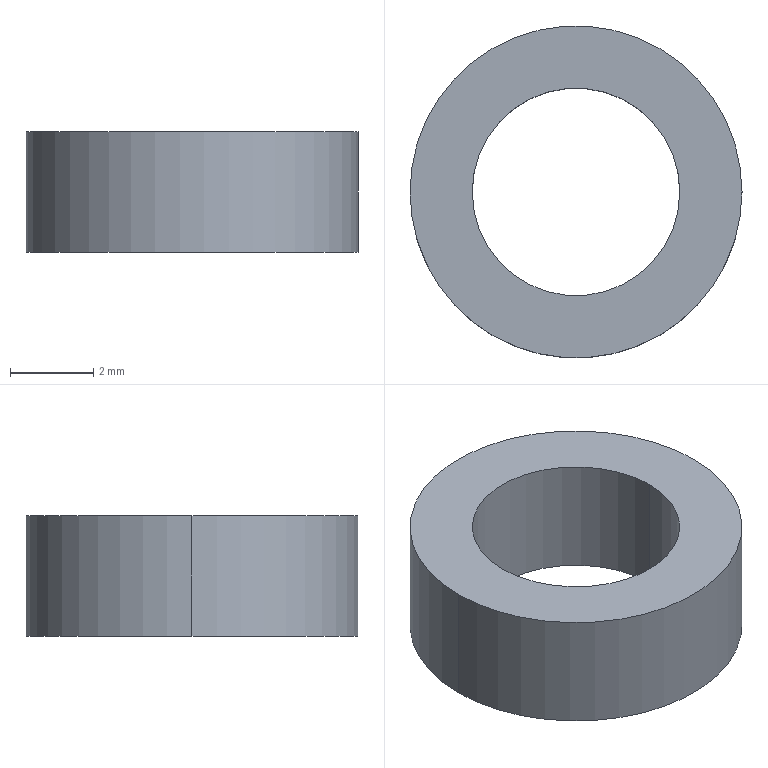Part | SolidWorks | features Extrusion 1 | 1 solid | 6 faces | box 8 x 8 x 2.9 mm | volume 88.829 mm3 | cylinder 4 | plane 2 | commonest cylinder face diameters 5 x2 8 x2
STEP:
#1=CARTESIAN_POINT('',(-2.5,0.,2.9));
#2=VERTEX_POINT('',#1);
#3=CARTESIAN_POINT('',(2.5,0.,2.9));
#4=VERTEX_POINT('',#3);
#5=CARTESIAN_POINT('',(0.,0.,2.9));
#6=DIRECTION('',(0.,0.,1.));
#7=DIRECTION('',(1.,0.,0.));
#8=AXIS2_PLACEMENT_3D('',#5,#6,#7);
#9=CIRCLE('',#8,2.5);
#10=EDGE_CURVE('',#2,#4,#9,.T.);
#11=ORIENTED_EDGE('',*,*,#10,.T.);
#12=CARTESIAN_POINT('',(2.5,0.,0.));
#13=VERTEX_POINT('',#12);
#14=CARTESIAN_POINT('',(2.5,0.,2.9));
#15=DIRECTION('',(0.,0.,-1.));
#16=VECTOR('',#15,1000.);
#17=LINE('',#14,#16);
#18=EDGE_CURVE('',#4,#13,#17,.T.);
#19=ORIENTED_EDGE('',*,*,#18,.T.);
#20=CARTESIAN_POINT('',(-2.5,0.,0.));
#21=VERTEX_POINT('',#20);
#22=CARTESIAN_POINT('',(0.,0.,0.));
#23=DIRECTION('',(0.,0.,1.));
#24=DIRECTION('',(1.,0.,0.));
#25=AXIS2_PLACEMENT_3D('',#22,#23,#24);
#26=CIRCLE('',#25,2.5);
#27=EDGE_CURVE('',#21,#13,#26,.T.);
#28=ORIENTED_EDGE('',*,*,#27,.F.);
#29=CARTESIAN_POINT('',(-2.5,0.,2.9));
#30=DIRECTION('',(0.,0.,-1.));
#31=VECTOR('',#30,1000.);
#32=LINE('',#29,#31);
#33=EDGE_CURVE('',#2,#21,#32,.T.);
#34=ORIENTED_EDGE('',*,*,#33,.F.);
#35=EDGE_LOOP('',(#11,#19,#28,#34));
#36=FACE_OUTER_BOUND('',#35,.T.);
#37=CARTESIAN_POINT('',(0.,0.,2.9));
#38=DIRECTION('',(0.,0.,-1.));
#39=DIRECTION('',(-1.,0.,0.));
#40=AXIS2_PLACEMENT_3D('',#37,#38,#39);
#41=CYLINDRICAL_SURFACE('',#40,2.5);
#42=ADVANCED_FACE('',(#36),#41,.F.);
#43=CARTESIAN_POINT('',(4.,0.,2.9));
#44=VERTEX_POINT('',#43);
#45=CARTESIAN_POINT('',(-4.,0.,2.9));
#46=VERTEX_POINT('',#45);
#47=CARTESIAN_POINT('',(0.,0.,2.9));
#48=DIRECTION('',(0.,0.,1.));
#49=DIRECTION('',(1.,0.,0.));
#50=AXIS2_PLACEMENT_3D('',#47,#48,#49);
#51=CIRCLE('',#50,4.);
#52=EDGE_CURVE('',#44,#46,#51,.T.);
#53=ORIENTED_EDGE('',*,*,#52,.F.);
#54=CARTESIAN_POINT('',(4.,0.,0.));
#55=VERTEX_POINT('',#54);
#56=CARTESIAN_POINT('',(4.,0.,2.9));
#57=DIRECTION('',(0.,0.,-1.));
#58=VECTOR('',#57,1000.);
#59=LINE('',#56,#58);
#60=EDGE_CURVE('',#44,#55,#59,.T.);
#61=ORIENTED_EDGE('',*,*,#60,.T.);
#62=CARTESIAN_POINT('',(-4.,0.,0.));
#63=VERTEX_POINT('',#62);
#64=CARTESIAN_POINT('',(0.,0.,0.));
#65=DIRECTION('',(0.,0.,1.));
#66=DIRECTION('',(1.,0.,0.));
#67=AXIS2_PLACEMENT_3D('',#64,#65,#66);
#68=CIRCLE('',#67,4.);
#69=EDGE_CURVE('',#55,#63,#68,.T.);
#70=ORIENTED_EDGE('',*,*,#69,.T.);
#71=CARTESIAN_POINT('',(-4.,0.,2.9));
#72=DIRECTION('',(0.,0.,-1.));
#73=VECTOR('',#72,1000.);
#74=LINE('',#71,#73);
#75=EDGE_CURVE('',#46,#63,#74,.T.);
#76=ORIENTED_EDGE('',*,*,#75,.F.);
#77=EDGE_LOOP('',(#53,#61,#70,#76));
#78=FACE_OUTER_BOUND('',#77,.T.);
#79=CARTESIAN_POINT('',(0.,0.,2.9));
#80=DIRECTION('',(0.,0.,-1.));
#81=DIRECTION('',(-1.,0.,0.));
#82=AXIS2_PLACEMENT_3D('',#79,#80,#81);
#83=CYLINDRICAL_SURFACE('',#82,4.);
#84=ADVANCED_FACE('',(#78),#83,.T.);
#85=CARTESIAN_POINT('',(0.,0.,2.9));
#86=DIRECTION('',(0.,0.,1.));
#87=DIRECTION('',(1.,0.,0.));
#88=AXIS2_PLACEMENT_3D('',#85,#86,#87);
#89=CIRCLE('',#88,4.);
#90=EDGE_CURVE('',#46,#44,#89,.T.);
#91=ORIENTED_EDGE('',*,*,#90,.T.);
#92=ORIENTED_EDGE('',*,*,#52,.T.);
#93=EDGE_LOOP('',(#91,#92));
#94=FACE_OUTER_BOUND('',#93,.T.);
#95=ORIENTED_EDGE('',*,*,#10,.F.);
#96=CARTESIAN_POINT('',(0.,0.,2.9));
#97=DIRECTION('',(0.,0.,1.));
#98=DIRECTION('',(1.,0.,0.));
#99=AXIS2_PLACEMENT_3D('',#96,#97,#98);
#100=CIRCLE('',#99,2.5);
#101=EDGE_CURVE('',#4,#2,#100,.T.);
#102=ORIENTED_EDGE('',*,*,#101,.F.);
#103=EDGE_LOOP('',(#95,#102));
#104=FACE_BOUND('',#103,.T.);
#105=CARTESIAN_POINT('',(0.,0.,2.9));
#106=DIRECTION('',(0.,0.,1.));
#107=DIRECTION('',(1.,0.,0.));
#108=AXIS2_PLACEMENT_3D('',#105,#106,#107);
#109=PLANE('',#108);
#110=ADVANCED_FACE('',(#94,#104),#109,.T.);
#111=CARTESIAN_POINT('',(0.,0.,0.));
#112=DIRECTION('',(0.,0.,1.));
#113=DIRECTION('',(1.,0.,0.));
#114=AXIS2_PLACEMENT_3D('',#111,#112,#113);
#115=CIRCLE('',#114,4.);
#116=EDGE_CURVE('',#63,#55,#115,.T.);
#117=ORIENTED_EDGE('',*,*,#116,.F.);
#118=ORIENTED_EDGE('',*,*,#69,.F.);
#119=EDGE_LOOP('',(#117,#118));
#120=FACE_OUTER_BOUND('',#119,.T.);
#121=ORIENTED_EDGE('',*,*,#27,.T.);
#122=CARTESIAN_POINT('',(0.,0.,0.));
#123=DIRECTION('',(0.,0.,1.));
#124=DIRECTION('',(1.,0.,0.));
#125=AXIS2_PLACEMENT_3D('',#122,#123,#124);
#126=CIRCLE('',#125,2.5);
#127=EDGE_CURVE('',#13,#21,#126,.T.);
#128=ORIENTED_EDGE('',*,*,#127,.T.);
#129=EDGE_LOOP('',(#121,#128));
#130=FACE_BOUND('',#129,.T.);
#131=CARTESIAN_POINT('',(0.,0.,0.));
#132=DIRECTION('',(0.,0.,1.));
#133=DIRECTION('',(1.,0.,0.));
#134=AXIS2_PLACEMENT_3D('',#131,#132,#133);
#135=PLANE('',#134);
#136=ADVANCED_FACE('',(#120,#130),#135,.F.);
#137=ORIENTED_EDGE('',*,*,#60,.F.);
#138=ORIENTED_EDGE('',*,*,#90,.F.);
#139=ORIENTED_EDGE('',*,*,#75,.T.);
#140=ORIENTED_EDGE('',*,*,#116,.T.);
#141=EDGE_LOOP('',(#137,#138,#139,#140));
#142=FACE_OUTER_BOUND('',#141,.T.);
#143=CARTESIAN_POINT('',(0.,0.,2.9));
#144=DIRECTION('',(0.,0.,-1.));
#145=DIRECTION('',(-1.,0.,0.));
#146=AXIS2_PLACEMENT_3D('',#143,#144,#145);
#147=CYLINDRICAL_SURFACE('',#146,4.);
#148=ADVANCED_FACE('',(#142),#147,.T.);
#149=ORIENTED_EDGE('',*,*,#18,.F.);
#150=ORIENTED_EDGE('',*,*,#101,.T.);
#151=ORIENTED_EDGE('',*,*,#33,.T.);
#152=ORIENTED_EDGE('',*,*,#127,.F.);
#153=EDGE_LOOP('',(#149,#150,#151,#152));
#154=FACE_OUTER_BOUND('',#153,.T.);
#155=CARTESIAN_POINT('',(0.,0.,2.9));
#156=DIRECTION('',(0.,0.,-1.));
#157=DIRECTION('',(-1.,0.,0.));
#158=AXIS2_PLACEMENT_3D('',#155,#156,#157);
#159=CYLINDRICAL_SURFACE('',#158,2.5);
#160=ADVANCED_FACE('',(#154),#159,.F.);
#161=CLOSED_SHELL('',(#42,#84,#110,#136,#148,#160));
#162=MANIFOLD_SOLID_BREP('',#161);
#163=CARTESIAN_POINT('',(0.,0.,0.));
#164=DIRECTION('',(0.,0.,1.));
#165=DIRECTION('',(1.,0.,0.));
#166=AXIS2_PLACEMENT_3D('',#163,#164,#165);
#167=(LENGTH_UNIT()NAMED_UNIT(*)SI_UNIT(.MILLI.,.METRE.));
#168=UNCERTAINTY_MEASURE_WITH_UNIT(LENGTH_MEASURE(0.00001),#167,'','');
#169=(NAMED_UNIT(*)PLANE_ANGLE_UNIT()SI_UNIT($,.RADIAN.));
#170=(NAMED_UNIT(*)SI_UNIT($,.STERADIAN.)SOLID_ANGLE_UNIT());
#171=(GEOMETRIC_REPRESENTATION_CONTEXT(3)GLOBAL_UNCERTAINTY_ASSIGNED_CONTEXT((#168))GLOBAL_UNIT_ASSIGNED_CONTEXT((#167,#169,#170))REPRESENTATION_CONTEXT('',''));
#172=ADVANCED_BREP_SHAPE_REPRESENTATION('',(#162,#166),#171);